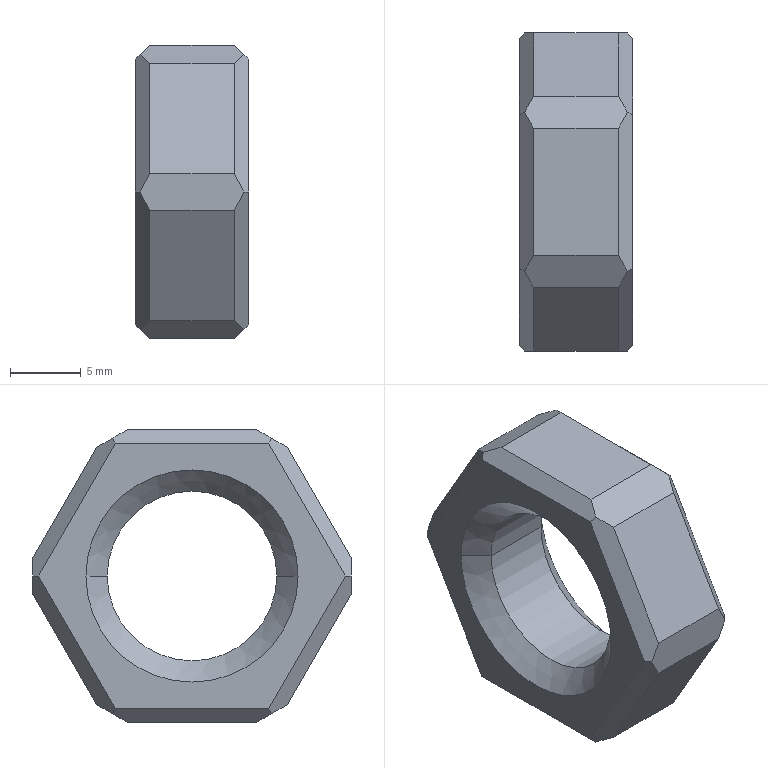Part | STEP file | PN_0019 | 1 solid | 32 faces | box 8 x 22.5 x 20.785 mm | volume 1889 mm3 | plane 26 | cone 4 | cylinder 2 | commonest cylinder face diameters 12 x2